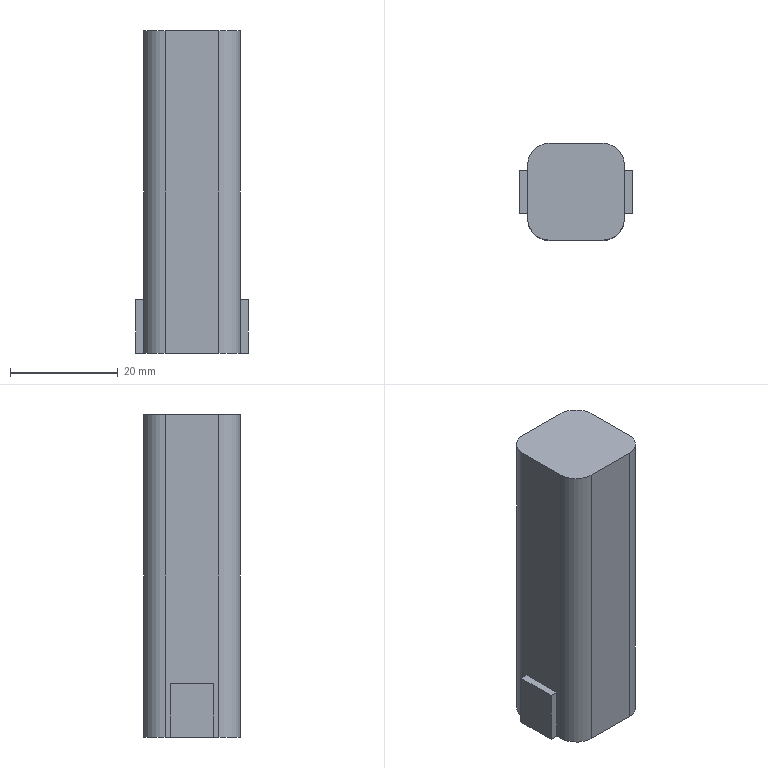Part | NX | features solid 2 | 1 solid | 18 faces | box 21 x 18 x 60 mm | volume 18856 mm3 | plane 14 | cylinder 4 | commonest cylinder face diameters 8 x4
STEP:
#1=CARTESIAN_POINT('',(1945.,111.,-68.));
#2=VERTEX_POINT('',#1);
#3=CARTESIAN_POINT('',(1945.,119.,-68.));
#4=VERTEX_POINT('',#3);
#5=CARTESIAN_POINT('',(1945.,115.,-68.));
#6=DIRECTION('',(0.,1.,0.));
#7=VECTOR('',#6,1000.);
#8=LINE('',#5,#7);
#9=EDGE_CURVE('',#2,#4,#8,.T.);
#10=ORIENTED_EDGE('',*,*,#9,.T.);
#11=CARTESIAN_POINT('',(1945.,119.,-78.));
#12=VERTEX_POINT('',#11);
#13=CARTESIAN_POINT('',(1945.,119.,-63.));
#14=DIRECTION('',(0.,0.,-1.));
#15=VECTOR('',#14,1000.);
#16=LINE('',#13,#15);
#17=EDGE_CURVE('',#4,#12,#16,.T.);
#18=ORIENTED_EDGE('',*,*,#17,.T.);
#19=CARTESIAN_POINT('',(1945.,120.,-78.));
#20=VERTEX_POINT('',#19);
#21=CARTESIAN_POINT('',(1945.,115.,-78.));
#22=DIRECTION('',(0.,-1.,0.));
#23=VECTOR('',#22,1000.);
#24=LINE('',#21,#23);
#25=EDGE_CURVE('',#20,#12,#24,.T.);
#26=ORIENTED_EDGE('',*,*,#25,.F.);
#27=CARTESIAN_POINT('',(1945.,120.,-18.));
#28=VERTEX_POINT('',#27);
#29=CARTESIAN_POINT('',(1945.,120.,-63.));
#30=DIRECTION('',(0.,0.,1.));
#31=VECTOR('',#30,1000.);
#32=LINE('',#29,#31);
#33=EDGE_CURVE('',#20,#28,#32,.T.);
#34=ORIENTED_EDGE('',*,*,#33,.T.);
#35=CARTESIAN_POINT('',(1945.,110.,-18.));
#36=VERTEX_POINT('',#35);
#37=CARTESIAN_POINT('',(1945.,115.,-18.));
#38=DIRECTION('',(0.,-1.,0.000000004));
#39=VECTOR('',#38,1000.);
#40=LINE('',#37,#39);
#41=EDGE_CURVE('',#28,#36,#40,.T.);
#42=ORIENTED_EDGE('',*,*,#41,.T.);
#43=CARTESIAN_POINT('',(1945.,110.,-78.));
#44=VERTEX_POINT('',#43);
#45=CARTESIAN_POINT('',(1945.,110.,-63.));
#46=DIRECTION('',(0.,0.,-1.));
#47=VECTOR('',#46,1000.);
#48=LINE('',#45,#47);
#49=EDGE_CURVE('',#36,#44,#48,.T.);
#50=ORIENTED_EDGE('',*,*,#49,.T.);
#51=CARTESIAN_POINT('',(1945.,111.,-78.));
#52=VERTEX_POINT('',#51);
#53=CARTESIAN_POINT('',(1945.,115.,-78.));
#54=DIRECTION('',(0.,-1.,0.));
#55=VECTOR('',#54,1000.);
#56=LINE('',#53,#55);
#57=EDGE_CURVE('',#52,#44,#56,.T.);
#58=ORIENTED_EDGE('',*,*,#57,.F.);
#59=CARTESIAN_POINT('',(1945.,111.,-63.));
#60=DIRECTION('',(0.,0.,1.));
#61=VECTOR('',#60,1000.);
#62=LINE('',#59,#61);
#63=EDGE_CURVE('',#52,#2,#62,.T.);
#64=ORIENTED_EDGE('',*,*,#63,.T.);
#65=EDGE_LOOP('',(#10,#18,#26,#34,#42,#50,#58,#64));
#66=FACE_BOUND('',#65,.T.);
#67=CARTESIAN_POINT('',(1945.,115.,-63.));
#68=DIRECTION('',(1.,0.,0.));
#69=DIRECTION('',(0.,0.,1.));
#70=AXIS2_PLACEMENT_3D('',#67,#68,#69);
#71=PLANE('',#70);
#72=ADVANCED_FACE('',(#66),#71,.T.);
#73=CARTESIAN_POINT('',(1927.,110.,-18.));
#74=VERTEX_POINT('',#73);
#75=CARTESIAN_POINT('',(1927.,120.,-18.));
#76=VERTEX_POINT('',#75);
#77=CARTESIAN_POINT('',(1927.,115.,-18.));
#78=DIRECTION('',(0.,1.,-0.000000004));
#79=VECTOR('',#78,1000.);
#80=LINE('',#77,#79);
#81=EDGE_CURVE('',#74,#76,#80,.T.);
#82=ORIENTED_EDGE('',*,*,#81,.F.);
#83=CARTESIAN_POINT('',(1931.,106.,-18.));
#84=VERTEX_POINT('',#83);
#85=CARTESIAN_POINT('',(1931.,110.,-18.));
#86=DIRECTION('',(0.,0.000000004,1.));
#87=DIRECTION('',(0.,-1.,0.000000004));
#88=AXIS2_PLACEMENT_3D('',#85,#86,#87);
#89=CIRCLE('',#88,4.);
#90=EDGE_CURVE('',#74,#84,#89,.T.);
#91=ORIENTED_EDGE('',*,*,#90,.T.);
#92=CARTESIAN_POINT('',(1941.,106.,-18.));
#93=VERTEX_POINT('',#92);
#94=CARTESIAN_POINT('',(1936.,106.,-18.));
#95=DIRECTION('',(-1.,0.,0.));
#96=VECTOR('',#95,1000.);
#97=LINE('',#94,#96);
#98=EDGE_CURVE('',#93,#84,#97,.T.);
#99=ORIENTED_EDGE('',*,*,#98,.F.);
#100=CARTESIAN_POINT('',(1941.,110.,-18.));
#101=DIRECTION('',(0.,0.000000004,1.));
#102=DIRECTION('',(0.,-1.,0.000000004));
#103=AXIS2_PLACEMENT_3D('',#100,#101,#102);
#104=CIRCLE('',#103,4.);
#105=EDGE_CURVE('',#93,#36,#104,.T.);
#106=ORIENTED_EDGE('',*,*,#105,.T.);
#107=ORIENTED_EDGE('',*,*,#41,.F.);
#108=CARTESIAN_POINT('',(1941.,124.,-18.));
#109=VERTEX_POINT('',#108);
#110=CARTESIAN_POINT('',(1941.,120.,-18.));
#111=DIRECTION('',(0.,0.000000004,1.));
#112=DIRECTION('',(0.,-1.,0.000000004));
#113=AXIS2_PLACEMENT_3D('',#110,#111,#112);
#114=CIRCLE('',#113,4.);
#115=EDGE_CURVE('',#28,#109,#114,.T.);
#116=ORIENTED_EDGE('',*,*,#115,.T.);
#117=CARTESIAN_POINT('',(1931.,124.,-18.));
#118=VERTEX_POINT('',#117);
#119=CARTESIAN_POINT('',(1936.,124.,-18.));
#120=DIRECTION('',(1.,0.,0.));
#121=VECTOR('',#120,1000.);
#122=LINE('',#119,#121);
#123=EDGE_CURVE('',#118,#109,#122,.T.);
#124=ORIENTED_EDGE('',*,*,#123,.F.);
#125=CARTESIAN_POINT('',(1931.,120.,-18.));
#126=DIRECTION('',(0.,0.000000004,1.));
#127=DIRECTION('',(0.,-1.,0.000000004));
#128=AXIS2_PLACEMENT_3D('',#125,#126,#127);
#129=CIRCLE('',#128,4.);
#130=EDGE_CURVE('',#118,#76,#129,.T.);
#131=ORIENTED_EDGE('',*,*,#130,.T.);
#132=EDGE_LOOP('',(#82,#91,#99,#106,#107,#116,#124,#131));
#133=FACE_BOUND('',#132,.T.);
#134=CARTESIAN_POINT('',(1872.159,111.584,-18.));
#135=DIRECTION('',(0.,0.000000004,1.));
#136=DIRECTION('',(-0.9367,0.3502,-0.000000001));
#137=AXIS2_PLACEMENT_3D('',#134,#135,#136);
#138=PLANE('',#137);
#139=ADVANCED_FACE('',(#133),#138,.T.);
#140=CARTESIAN_POINT('',(1931.,106.,-78.));
#141=VERTEX_POINT('',#140);
#142=CARTESIAN_POINT('',(1941.,106.,-78.));
#143=VERTEX_POINT('',#142);
#144=CARTESIAN_POINT('',(1936.,106.,-78.));
#145=DIRECTION('',(1.,0.,0.));
#146=VECTOR('',#145,1000.);
#147=LINE('',#144,#146);
#148=EDGE_CURVE('',#141,#143,#147,.T.);
#149=ORIENTED_EDGE('',*,*,#148,.T.);
#150=CARTESIAN_POINT('',(1941.,106.,-63.));
#151=DIRECTION('',(0.,0.,1.));
#152=VECTOR('',#151,1000.);
#153=LINE('',#150,#152);
#154=EDGE_CURVE('',#143,#93,#153,.T.);
#155=ORIENTED_EDGE('',*,*,#154,.T.);
#156=ORIENTED_EDGE('',*,*,#98,.T.);
#157=CARTESIAN_POINT('',(1931.,106.,-63.));
#158=DIRECTION('',(0.,0.,-1.));
#159=VECTOR('',#158,1000.);
#160=LINE('',#157,#159);
#161=EDGE_CURVE('',#84,#141,#160,.T.);
#162=ORIENTED_EDGE('',*,*,#161,.T.);
#163=EDGE_LOOP('',(#149,#155,#156,#162));
#164=FACE_BOUND('',#163,.T.);
#165=CARTESIAN_POINT('',(1936.,106.,-63.));
#166=DIRECTION('',(0.,-1.,0.));
#167=DIRECTION('',(0.,0.,1.));
#168=AXIS2_PLACEMENT_3D('',#165,#166,#167);
#169=PLANE('',#168);
#170=ADVANCED_FACE('',(#164),#169,.T.);
#171=CARTESIAN_POINT('',(1927.,111.,-78.));
#172=VERTEX_POINT('',#171);
#173=CARTESIAN_POINT('',(1927.,111.,-68.));
#174=VERTEX_POINT('',#173);
#175=CARTESIAN_POINT('',(1927.,111.,-63.));
#176=DIRECTION('',(0.,0.,1.));
#177=VECTOR('',#176,1000.);
#178=LINE('',#175,#177);
#179=EDGE_CURVE('',#172,#174,#178,.T.);
#180=ORIENTED_EDGE('',*,*,#179,.F.);
#181=CARTESIAN_POINT('',(1927.,110.,-78.));
#182=VERTEX_POINT('',#181);
#183=CARTESIAN_POINT('',(1927.,115.,-78.));
#184=DIRECTION('',(0.,1.,0.));
#185=VECTOR('',#184,1000.);
#186=LINE('',#183,#185);
#187=EDGE_CURVE('',#182,#172,#186,.T.);
#188=ORIENTED_EDGE('',*,*,#187,.F.);
#189=CARTESIAN_POINT('',(1927.,110.,-63.));
#190=DIRECTION('',(0.,0.,1.));
#191=VECTOR('',#190,1000.);
#192=LINE('',#189,#191);
#193=EDGE_CURVE('',#182,#74,#192,.T.);
#194=ORIENTED_EDGE('',*,*,#193,.T.);
#195=ORIENTED_EDGE('',*,*,#81,.T.);
#196=CARTESIAN_POINT('',(1927.,120.,-78.));
#197=VERTEX_POINT('',#196);
#198=CARTESIAN_POINT('',(1927.,120.,-63.));
#199=DIRECTION('',(0.,0.,-1.));
#200=VECTOR('',#199,1000.);
#201=LINE('',#198,#200);
#202=EDGE_CURVE('',#76,#197,#201,.T.);
#203=ORIENTED_EDGE('',*,*,#202,.T.);
#204=CARTESIAN_POINT('',(1927.,119.,-78.));
#205=VERTEX_POINT('',#204);
#206=CARTESIAN_POINT('',(1927.,115.,-78.));
#207=DIRECTION('',(0.,1.,0.));
#208=VECTOR('',#207,1000.);
#209=LINE('',#206,#208);
#210=EDGE_CURVE('',#205,#197,#209,.T.);
#211=ORIENTED_EDGE('',*,*,#210,.F.);
#212=CARTESIAN_POINT('',(1927.,119.,-68.));
#213=VERTEX_POINT('',#212);
#214=CARTESIAN_POINT('',(1927.,119.,-63.));
#215=DIRECTION('',(0.,0.,-1.));
#216=VECTOR('',#215,1000.);
#217=LINE('',#214,#216);
#218=EDGE_CURVE('',#213,#205,#217,.T.);
#219=ORIENTED_EDGE('',*,*,#218,.F.);
#220=CARTESIAN_POINT('',(1927.,115.,-68.));
#221=DIRECTION('',(0.,1.,0.));
#222=VECTOR('',#221,1000.);
#223=LINE('',#220,#222);
#224=EDGE_CURVE('',#174,#213,#223,.T.);
#225=ORIENTED_EDGE('',*,*,#224,.F.);
#226=EDGE_LOOP('',(#180,#188,#194,#195,#203,#211,#219,#225));
#227=FACE_BOUND('',#226,.T.);
#228=CARTESIAN_POINT('',(1927.,115.,-63.));
#229=DIRECTION('',(-1.,0.,0.));
#230=DIRECTION('',(0.,0.,-1.));
#231=AXIS2_PLACEMENT_3D('',#228,#229,#230);
#232=PLANE('',#231);
#233=ADVANCED_FACE('',(#227),#232,.T.);
#234=CARTESIAN_POINT('',(1941.,124.,-78.));
#235=VERTEX_POINT('',#234);
#236=CARTESIAN_POINT('',(1931.,124.,-78.));
#237=VERTEX_POINT('',#236);
#238=CARTESIAN_POINT('',(1936.,124.,-78.));
#239=DIRECTION('',(-1.,0.,0.));
#240=VECTOR('',#239,1000.);
#241=LINE('',#238,#240);
#242=EDGE_CURVE('',#235,#237,#241,.T.);
#243=ORIENTED_EDGE('',*,*,#242,.T.);
#244=CARTESIAN_POINT('',(1931.,124.,-63.));
#245=DIRECTION('',(0.,0.,1.));
#246=VECTOR('',#245,1000.);
#247=LINE('',#244,#246);
#248=EDGE_CURVE('',#237,#118,#247,.T.);
#249=ORIENTED_EDGE('',*,*,#248,.T.);
#250=ORIENTED_EDGE('',*,*,#123,.T.);
#251=CARTESIAN_POINT('',(1941.,124.,-63.));
#252=DIRECTION('',(0.,0.,-1.));
#253=VECTOR('',#252,1000.);
#254=LINE('',#251,#253);
#255=EDGE_CURVE('',#109,#235,#254,.T.);
#256=ORIENTED_EDGE('',*,*,#255,.T.);
#257=EDGE_LOOP('',(#243,#249,#250,#256));
#258=FACE_BOUND('',#257,.T.);
#259=CARTESIAN_POINT('',(1936.,124.,-63.));
#260=DIRECTION('',(0.,1.,0.));
#261=DIRECTION('',(0.,0.,-1.));
#262=AXIS2_PLACEMENT_3D('',#259,#260,#261);
#263=PLANE('',#262);
#264=ADVANCED_FACE('',(#258),#263,.T.);
#265=CARTESIAN_POINT('',(1931.,110.,-78.));
#266=DIRECTION('',(0.,0.,-1.));
#267=DIRECTION('',(-1.,0.,0.));
#268=AXIS2_PLACEMENT_3D('',#265,#266,#267);
#269=CIRCLE('',#268,4.);
#270=EDGE_CURVE('',#141,#182,#269,.T.);
#271=ORIENTED_EDGE('',*,*,#270,.F.);
#272=ORIENTED_EDGE('',*,*,#161,.F.);
#273=ORIENTED_EDGE('',*,*,#90,.F.);
#274=ORIENTED_EDGE('',*,*,#193,.F.);
#275=EDGE_LOOP('',(#271,#272,#273,#274));
#276=FACE_BOUND('',#275,.T.);
#277=CARTESIAN_POINT('',(1931.,110.,-63.));
#278=DIRECTION('',(0.,0.,1.));
#279=DIRECTION('',(-1.,0.,0.));
#280=AXIS2_PLACEMENT_3D('',#277,#278,#279);
#281=CYLINDRICAL_SURFACE('',#280,4.);
#282=ADVANCED_FACE('',(#276),#281,.T.);
#283=CARTESIAN_POINT('',(1941.,110.,-78.));
#284=DIRECTION('',(0.,0.,-1.));
#285=DIRECTION('',(-1.,0.,0.));
#286=AXIS2_PLACEMENT_3D('',#283,#284,#285);
#287=CIRCLE('',#286,4.);
#288=EDGE_CURVE('',#44,#143,#287,.T.);
#289=ORIENTED_EDGE('',*,*,#288,.F.);
#290=ORIENTED_EDGE('',*,*,#49,.F.);
#291=ORIENTED_EDGE('',*,*,#105,.F.);
#292=ORIENTED_EDGE('',*,*,#154,.F.);
#293=EDGE_LOOP('',(#289,#290,#291,#292));
#294=FACE_BOUND('',#293,.T.);
#295=CARTESIAN_POINT('',(1941.,110.,-63.));
#296=DIRECTION('',(0.,0.,1.));
#297=DIRECTION('',(-1.,0.,0.));
#298=AXIS2_PLACEMENT_3D('',#295,#296,#297);
#299=CYLINDRICAL_SURFACE('',#298,4.);
#300=ADVANCED_FACE('',(#294),#299,.T.);
#301=CARTESIAN_POINT('',(1941.,120.,-78.));
#302=DIRECTION('',(0.,0.,-1.));
#303=DIRECTION('',(-1.,0.,0.));
#304=AXIS2_PLACEMENT_3D('',#301,#302,#303);
#305=CIRCLE('',#304,4.);
#306=EDGE_CURVE('',#235,#20,#305,.T.);
#307=ORIENTED_EDGE('',*,*,#306,.F.);
#308=ORIENTED_EDGE('',*,*,#255,.F.);
#309=ORIENTED_EDGE('',*,*,#115,.F.);
#310=ORIENTED_EDGE('',*,*,#33,.F.);
#311=EDGE_LOOP('',(#307,#308,#309,#310));
#312=FACE_BOUND('',#311,.T.);
#313=CARTESIAN_POINT('',(1941.,120.,-63.));
#314=DIRECTION('',(0.,0.,1.));
#315=DIRECTION('',(-1.,0.,0.));
#316=AXIS2_PLACEMENT_3D('',#313,#314,#315);
#317=CYLINDRICAL_SURFACE('',#316,4.);
#318=ADVANCED_FACE('',(#312),#317,.T.);
#319=CARTESIAN_POINT('',(1931.,120.,-78.));
#320=DIRECTION('',(0.,0.,-1.));
#321=DIRECTION('',(-1.,0.,0.));
#322=AXIS2_PLACEMENT_3D('',#319,#320,#321);
#323=CIRCLE('',#322,4.);
#324=EDGE_CURVE('',#197,#237,#323,.T.);
#325=ORIENTED_EDGE('',*,*,#324,.F.);
#326=ORIENTED_EDGE('',*,*,#202,.F.);
#327=ORIENTED_EDGE('',*,*,#130,.F.);
#328=ORIENTED_EDGE('',*,*,#248,.F.);
#329=EDGE_LOOP('',(#325,#326,#327,#328));
#330=FACE_BOUND('',#329,.T.);
#331=CARTESIAN_POINT('',(1931.,120.,-63.));
#332=DIRECTION('',(0.,0.,1.));
#333=DIRECTION('',(-1.,0.,0.));
#334=AXIS2_PLACEMENT_3D('',#331,#332,#333);
#335=CYLINDRICAL_SURFACE('',#334,4.);
#336=ADVANCED_FACE('',(#330),#335,.T.);
#337=ORIENTED_EDGE('',*,*,#306,.T.);
#338=ORIENTED_EDGE('',*,*,#25,.T.);
#339=CARTESIAN_POINT('',(1946.5,119.,-78.));
#340=VERTEX_POINT('',#339);
#341=CARTESIAN_POINT('',(1946.5,119.,-78.));
#342=DIRECTION('',(-1.,0.,0.));
#343=VECTOR('',#342,1000.);
#344=LINE('',#341,#343);
#345=EDGE_CURVE('',#340,#12,#344,.T.);
#346=ORIENTED_EDGE('',*,*,#345,.F.);
#347=CARTESIAN_POINT('',(1946.5,111.,-78.));
#348=VERTEX_POINT('',#347);
#349=CARTESIAN_POINT('',(1946.5,115.,-78.));
#350=DIRECTION('',(0.,1.,0.));
#351=VECTOR('',#350,1000.);
#352=LINE('',#349,#351);
#353=EDGE_CURVE('',#348,#340,#352,.T.);
#354=ORIENTED_EDGE('',*,*,#353,.F.);
#355=CARTESIAN_POINT('',(1946.5,111.,-78.));
#356=DIRECTION('',(-1.,0.,0.));
#357=VECTOR('',#356,1000.);
#358=LINE('',#355,#357);
#359=EDGE_CURVE('',#348,#52,#358,.T.);
#360=ORIENTED_EDGE('',*,*,#359,.T.);
#361=ORIENTED_EDGE('',*,*,#57,.T.);
#362=ORIENTED_EDGE('',*,*,#288,.T.);
#363=ORIENTED_EDGE('',*,*,#148,.F.);
#364=ORIENTED_EDGE('',*,*,#270,.T.);
#365=ORIENTED_EDGE('',*,*,#187,.T.);
#366=CARTESIAN_POINT('',(1925.5,111.,-78.));
#367=VERTEX_POINT('',#366);
#368=CARTESIAN_POINT('',(1925.5,111.,-78.));
#369=DIRECTION('',(1.,0.,0.));
#370=VECTOR('',#369,1000.);
#371=LINE('',#368,#370);
#372=EDGE_CURVE('',#367,#172,#371,.T.);
#373=ORIENTED_EDGE('',*,*,#372,.F.);
#374=CARTESIAN_POINT('',(1925.5,119.,-78.));
#375=VERTEX_POINT('',#374);
#376=CARTESIAN_POINT('',(1925.5,115.,-78.));
#377=DIRECTION('',(0.,1.,0.));
#378=VECTOR('',#377,1000.);
#379=LINE('',#376,#378);
#380=EDGE_CURVE('',#367,#375,#379,.T.);
#381=ORIENTED_EDGE('',*,*,#380,.T.);
#382=CARTESIAN_POINT('',(1925.5,119.,-78.));
#383=DIRECTION('',(1.,0.,0.));
#384=VECTOR('',#383,1000.);
#385=LINE('',#382,#384);
#386=EDGE_CURVE('',#375,#205,#385,.T.);
#387=ORIENTED_EDGE('',*,*,#386,.T.);
#388=ORIENTED_EDGE('',*,*,#210,.T.);
#389=ORIENTED_EDGE('',*,*,#324,.T.);
#390=ORIENTED_EDGE('',*,*,#242,.F.);
#391=EDGE_LOOP('',(#337,#338,#346,#354,#360,#361,#362,#363,#364,#365,#373,#381,#387,#388,#389,#390));
#392=FACE_BOUND('',#391,.T.);
#393=CARTESIAN_POINT('',(1936.,115.,-78.));
#394=DIRECTION('',(0.,0.,-1.));
#395=DIRECTION('',(1.,0.,0.));
#396=AXIS2_PLACEMENT_3D('',#393,#394,#395);
#397=PLANE('',#396);
#398=ADVANCED_FACE('',(#392),#397,.T.);
#399=CARTESIAN_POINT('',(1925.5,111.,-68.));
#400=VERTEX_POINT('',#399);
#401=CARTESIAN_POINT('',(1925.5,111.,-68.));
#402=DIRECTION('',(1.,0.,0.));
#403=VECTOR('',#402,1000.);
#404=LINE('',#401,#403);
#405=EDGE_CURVE('',#400,#174,#404,.T.);
#406=ORIENTED_EDGE('',*,*,#405,.F.);
#407=CARTESIAN_POINT('',(1925.5,111.,-63.));
#408=DIRECTION('',(0.,0.,1.));
#409=VECTOR('',#408,1000.);
#410=LINE('',#407,#409);
#411=EDGE_CURVE('',#367,#400,#410,.T.);
#412=ORIENTED_EDGE('',*,*,#411,.F.);
#413=ORIENTED_EDGE('',*,*,#372,.T.);
#414=ORIENTED_EDGE('',*,*,#179,.T.);
#415=EDGE_LOOP('',(#406,#412,#413,#414));
#416=FACE_BOUND('',#415,.T.);
#417=CARTESIAN_POINT('',(1925.5,111.,-63.));
#418=DIRECTION('',(0.,1.,0.));
#419=DIRECTION('',(0.,0.,-1.));
#420=AXIS2_PLACEMENT_3D('',#417,#418,#419);
#421=PLANE('',#420);
#422=ADVANCED_FACE('',(#416),#421,.F.);
#423=CARTESIAN_POINT('',(1925.5,119.,-68.));
#424=VERTEX_POINT('',#423);
#425=CARTESIAN_POINT('',(1925.5,119.,-68.));
#426=DIRECTION('',(-1.,0.,0.));
#427=VECTOR('',#426,1000.);
#428=LINE('',#425,#427);
#429=EDGE_CURVE('',#213,#424,#428,.T.);
#430=ORIENTED_EDGE('',*,*,#429,.F.);
#431=ORIENTED_EDGE('',*,*,#218,.T.);
#432=ORIENTED_EDGE('',*,*,#386,.F.);
#433=CARTESIAN_POINT('',(1925.5,119.,-63.));
#434=DIRECTION('',(0.,0.,-1.));
#435=VECTOR('',#434,1000.);
#436=LINE('',#433,#435);
#437=EDGE_CURVE('',#424,#375,#436,.T.);
#438=ORIENTED_EDGE('',*,*,#437,.F.);
#439=EDGE_LOOP('',(#430,#431,#432,#438));
#440=FACE_BOUND('',#439,.T.);
#441=CARTESIAN_POINT('',(1925.5,119.,-63.));
#442=DIRECTION('',(0.,-1.,0.));
#443=DIRECTION('',(0.,0.,1.));
#444=AXIS2_PLACEMENT_3D('',#441,#442,#443);
#445=PLANE('',#444);
#446=ADVANCED_FACE('',(#440),#445,.F.);
#447=ORIENTED_EDGE('',*,*,#411,.T.);
#448=CARTESIAN_POINT('',(1925.5,115.,-68.));
#449=DIRECTION('',(0.,1.,0.));
#450=VECTOR('',#449,1000.);
#451=LINE('',#448,#450);
#452=EDGE_CURVE('',#400,#424,#451,.T.);
#453=ORIENTED_EDGE('',*,*,#452,.T.);
#454=ORIENTED_EDGE('',*,*,#437,.T.);
#455=ORIENTED_EDGE('',*,*,#380,.F.);
#456=EDGE_LOOP('',(#447,#453,#454,#455));
#457=FACE_BOUND('',#456,.T.);
#458=CARTESIAN_POINT('',(1925.5,115.,-63.));
#459=DIRECTION('',(-1.,0.,0.));
#460=DIRECTION('',(0.,0.,-1.));
#461=AXIS2_PLACEMENT_3D('',#458,#459,#460);
#462=PLANE('',#461);
#463=ADVANCED_FACE('',(#457),#462,.T.);
#464=ORIENTED_EDGE('',*,*,#452,.F.);
#465=ORIENTED_EDGE('',*,*,#405,.T.);
#466=ORIENTED_EDGE('',*,*,#224,.T.);
#467=ORIENTED_EDGE('',*,*,#429,.T.);
#468=EDGE_LOOP('',(#464,#465,#466,#467));
#469=FACE_BOUND('',#468,.T.);
#470=CARTESIAN_POINT('',(1936.,115.,-68.));
#471=DIRECTION('',(0.,0.,1.));
#472=DIRECTION('',(-1.,0.,0.));
#473=AXIS2_PLACEMENT_3D('',#470,#471,#472);
#474=PLANE('',#473);
#475=ADVANCED_FACE('',(#469),#474,.T.);
#476=CARTESIAN_POINT('',(1946.5,111.,-68.));
#477=VERTEX_POINT('',#476);
#478=CARTESIAN_POINT('',(1946.5,111.,-68.));
#479=DIRECTION('',(-1.,0.,0.));
#480=VECTOR('',#479,1000.);
#481=LINE('',#478,#480);
#482=EDGE_CURVE('',#477,#2,#481,.T.);
#483=ORIENTED_EDGE('',*,*,#482,.T.);
#484=ORIENTED_EDGE('',*,*,#63,.F.);
#485=ORIENTED_EDGE('',*,*,#359,.F.);
#486=CARTESIAN_POINT('',(1946.5,111.,-63.));
#487=DIRECTION('',(0.,0.,1.));
#488=VECTOR('',#487,1000.);
#489=LINE('',#486,#488);
#490=EDGE_CURVE('',#348,#477,#489,.T.);
#491=ORIENTED_EDGE('',*,*,#490,.T.);
#492=EDGE_LOOP('',(#483,#484,#485,#491));
#493=FACE_BOUND('',#492,.T.);
#494=CARTESIAN_POINT('',(1946.5,111.,-63.));
#495=DIRECTION('',(0.,1.,0.));
#496=DIRECTION('',(0.,0.,-1.));
#497=AXIS2_PLACEMENT_3D('',#494,#495,#496);
#498=PLANE('',#497);
#499=ADVANCED_FACE('',(#493),#498,.F.);
#500=CARTESIAN_POINT('',(1946.5,119.,-68.));
#501=VERTEX_POINT('',#500);
#502=CARTESIAN_POINT('',(1946.5,119.,-68.));
#503=DIRECTION('',(1.,0.,0.));
#504=VECTOR('',#503,1000.);
#505=LINE('',#502,#504);
#506=EDGE_CURVE('',#4,#501,#505,.T.);
#507=ORIENTED_EDGE('',*,*,#506,.T.);
#508=CARTESIAN_POINT('',(1946.5,119.,-63.));
#509=DIRECTION('',(0.,0.,-1.));
#510=VECTOR('',#509,1000.);
#511=LINE('',#508,#510);
#512=EDGE_CURVE('',#501,#340,#511,.T.);
#513=ORIENTED_EDGE('',*,*,#512,.T.);
#514=ORIENTED_EDGE('',*,*,#345,.T.);
#515=ORIENTED_EDGE('',*,*,#17,.F.);
#516=EDGE_LOOP('',(#507,#513,#514,#515));
#517=FACE_BOUND('',#516,.T.);
#518=CARTESIAN_POINT('',(1946.5,119.,-63.));
#519=DIRECTION('',(0.,-1.,0.));
#520=DIRECTION('',(0.,0.,1.));
#521=AXIS2_PLACEMENT_3D('',#518,#519,#520);
#522=PLANE('',#521);
#523=ADVANCED_FACE('',(#517),#522,.F.);
#524=ORIENTED_EDGE('',*,*,#490,.F.);
#525=ORIENTED_EDGE('',*,*,#353,.T.);
#526=ORIENTED_EDGE('',*,*,#512,.F.);
#527=CARTESIAN_POINT('',(1946.5,115.,-68.));
#528=DIRECTION('',(0.,1.,0.));
#529=VECTOR('',#528,1000.);
#530=LINE('',#527,#529);
#531=EDGE_CURVE('',#477,#501,#530,.T.);
#532=ORIENTED_EDGE('',*,*,#531,.F.);
#533=EDGE_LOOP('',(#524,#525,#526,#532));
#534=FACE_BOUND('',#533,.T.);
#535=CARTESIAN_POINT('',(1946.5,115.,-63.));
#536=DIRECTION('',(1.,0.,0.));
#537=DIRECTION('',(0.,0.,-1.));
#538=AXIS2_PLACEMENT_3D('',#535,#536,#537);
#539=PLANE('',#538);
#540=ADVANCED_FACE('',(#534),#539,.T.);
#541=ORIENTED_EDGE('',*,*,#531,.T.);
#542=ORIENTED_EDGE('',*,*,#506,.F.);
#543=ORIENTED_EDGE('',*,*,#9,.F.);
#544=ORIENTED_EDGE('',*,*,#482,.F.);
#545=EDGE_LOOP('',(#541,#542,#543,#544));
#546=FACE_BOUND('',#545,.T.);
#547=CARTESIAN_POINT('',(1936.,115.,-68.));
#548=DIRECTION('',(0.,0.,1.));
#549=DIRECTION('',(1.,0.,0.));
#550=AXIS2_PLACEMENT_3D('',#547,#548,#549);
#551=PLANE('',#550);
#552=ADVANCED_FACE('',(#546),#551,.T.);
#553=CLOSED_SHELL('',(#72,#139,#170,#233,#264,#282,#300,#318,#336,#398,#422,#446,#463,#475,#499,#523,#540,#552));
#554=MANIFOLD_SOLID_BREP('',#553);
#555=(LENGTH_UNIT()NAMED_UNIT(*)SI_UNIT(.MILLI.,.METRE.));
#556=UNCERTAINTY_MEASURE_WITH_UNIT(LENGTH_MEASURE(0.00001),#555,'','');
#557=(NAMED_UNIT(*)PLANE_ANGLE_UNIT()SI_UNIT($,.RADIAN.));
#558=(NAMED_UNIT(*)SI_UNIT($,.STERADIAN.)SOLID_ANGLE_UNIT());
#559=(GEOMETRIC_REPRESENTATION_CONTEXT(3)GLOBAL_UNCERTAINTY_ASSIGNED_CONTEXT((#556))GLOBAL_UNIT_ASSIGNED_CONTEXT((#555,#557,#558))REPRESENTATION_CONTEXT('',''));
#560=ADVANCED_BREP_SHAPE_REPRESENTATION('',(#554),#559);